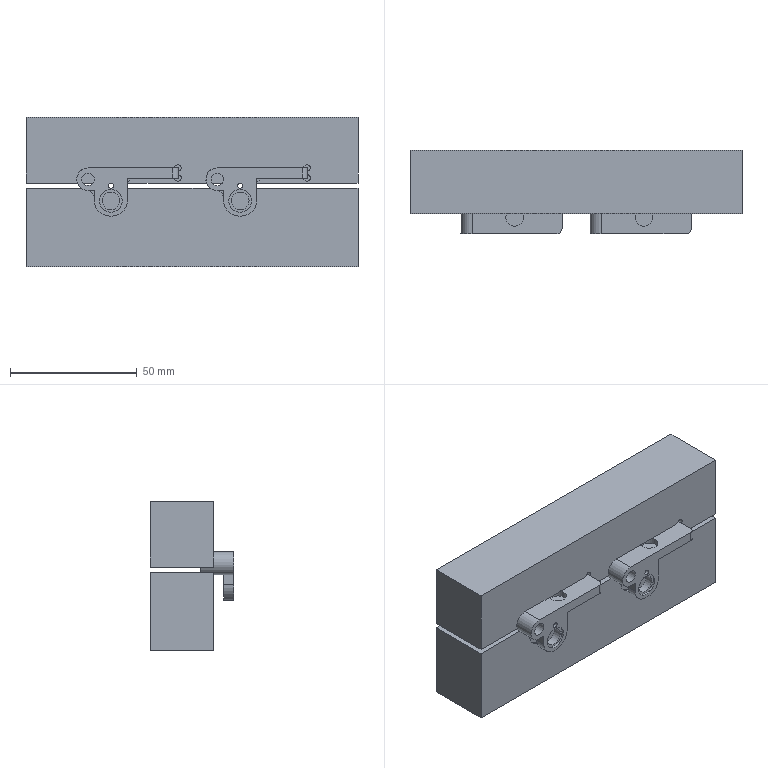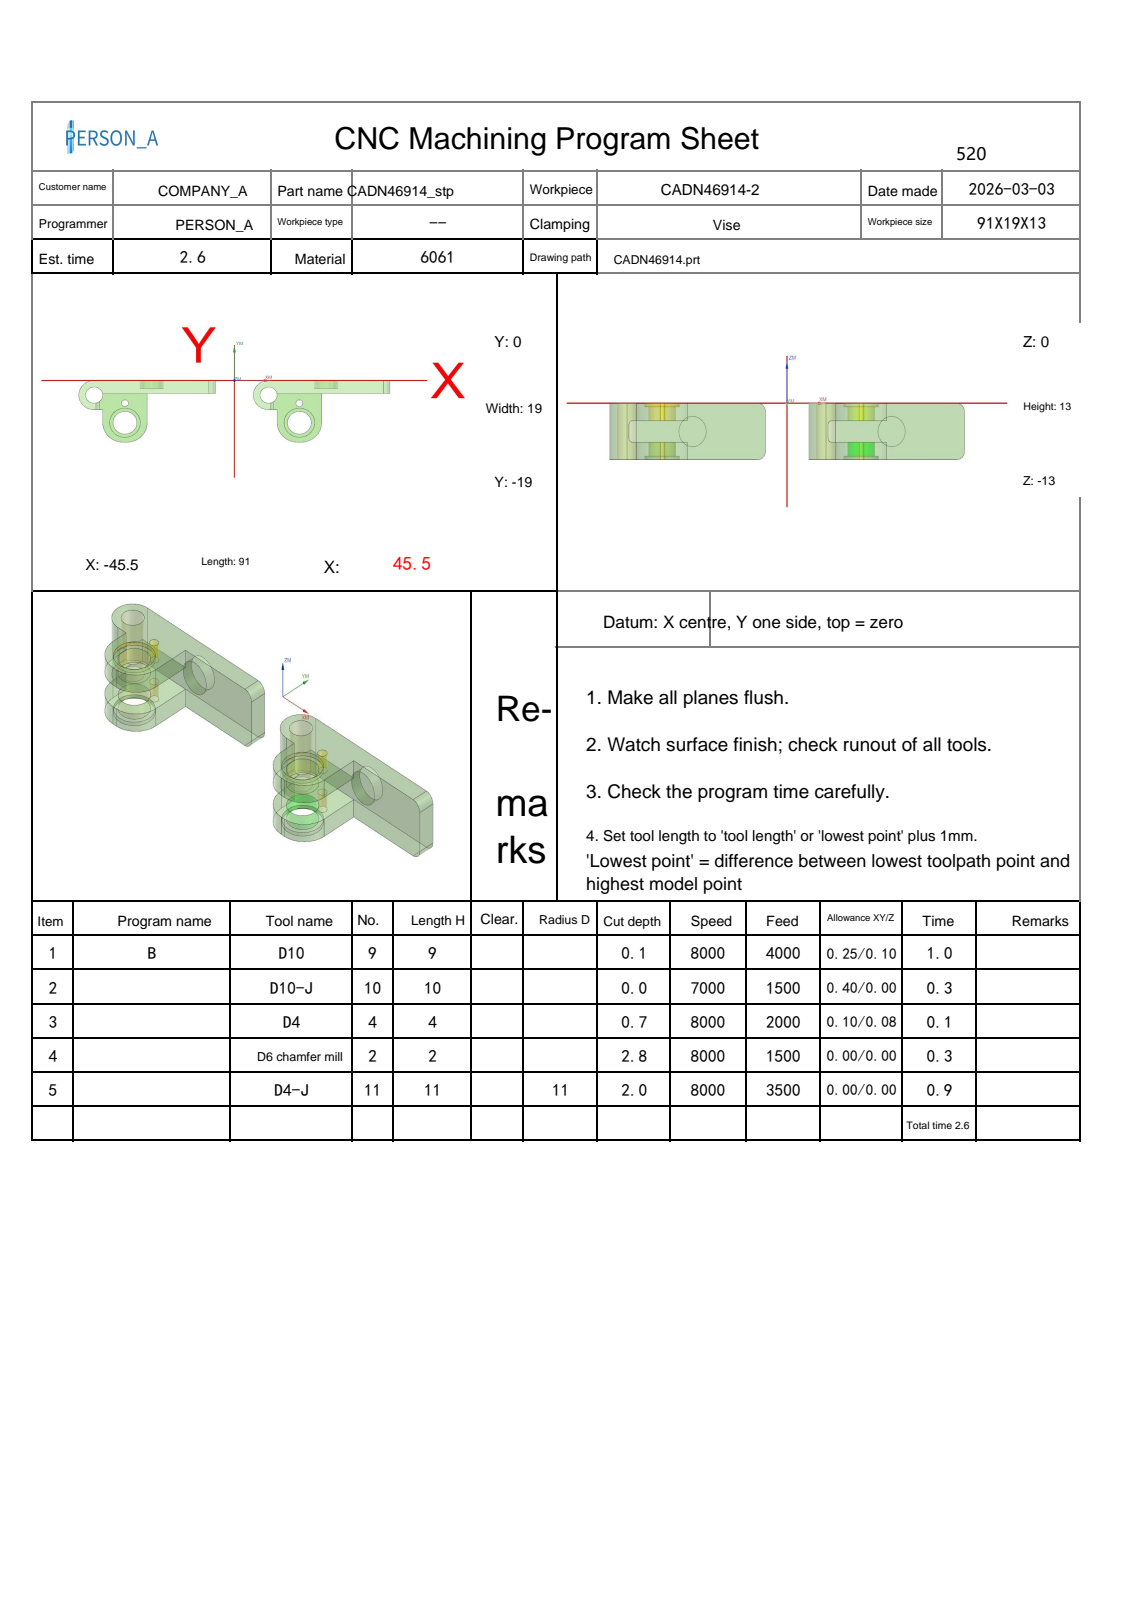NC program | NX | posted by the shop | part box 131 x 33 x 59 mm
Lines 824 to 1991 of 3834:
N5 T11 M06
(D4-J  D=4. R=0. H=11 ce=0.00 di=0.00)
G00 G90 G54 X20.661 Y-11.18 M03 S8000
G43 H11 Z50.
M08
Z.7
G01 X20.601 Y-11.119 Z.696 F600.
X20.28 Y-10.888 Z.675
X19.926 Y-10.71 Z.654
X19.549 Y-10.592 Z.633
X19.157 Y-10.535 Z.613
X18.843 Z.596
X18.451 Y-10.592 Z.575
X18.074 Y-10.71 Z.555
X17.72 Y-10.888 Z.534
X17.399 Y-11.119 Z.513
X17.119 Y-11.399 Z.492
X16.888 Y-11.72 Z.472
X16.71 Y-12.074 Z.451
X16.592 Y-12.451 Z.43
X16.535 Y-12.843 Z.409
Y-13.157 Z.393
X16.602 Y-13.593 Z.37
X16.746 Y-14.009 Z.347
X16.961 Y-14.394 Z.324
X17.241 Y-14.734 Z.301
X17.577 Y-15.019 Z.278
X17.959 Y-15.24 Z.254
X18.373 Y-15.389 Z.231
X18.808 Y-15.462 Z.208
X18.965 Y-15.465 Z.2
G41 D11
X19. Y-15.5
G03 X21.5 Y-13. Z-.05 I0.0 J2.5
X19. Y-10.5 Z-.3 I-2.5 J0.0
X16.5 Y-13. Z-.55 I0.0 J-2.5
X19. Y-15.5 Z-.8 I2.5 J0.0
X21.5 Y-13. I0.0 J2.5
X19. Y-10.5 I-2.5 J0.0
X16.5 Y-13. I0.0 J-2.5
X19. Y-15.5 I2.5 J0.0
X19.398 Y-15.468 I0.0 J2.5
G01 X19.425 Y-15.461
X19.442 Y-15.438
X19.44 Y-15.411
G40 X19.432 Y-15.361
Z.2
G00 Z50.
X-30.339 Y-11.18
Z.7
G01 X-30.399 Y-11.119 Z.696
X-30.72 Y-10.888 Z.675
X-31.074 Y-10.71 Z.654
X-31.451 Y-10.592 Z.633
X-31.843 Y-10.535 Z.613
X-32.157 Z.596
X-32.562 Y-10.595 Z.575
X-32.951 Y-10.721 Z.553
X-33.315 Y-10.909 Z.532
X-33.642 Y-11.155 Z.51
X-33.924 Y-11.452 Z.489
X-34.154 Y-11.791 Z.467
X-34.324 Y-12.163 Z.446
X-34.411 Y-12.465 Z.429
X-34.465 Y-12.843 Z.409
Y-13.157 Z.393
X-34.398 Y-13.593 Z.37
X-34.254 Y-14.009 Z.347
X-34.039 Y-14.394 Z.324
X-33.759 Y-14.734 Z.301
X-33.423 Y-15.019 Z.278
X-33.041 Y-15.24 Z.254
X-32.627 Y-15.389 Z.231
X-32.192 Y-15.462 Z.208
X-32.035 Y-15.465 Z.2
G41 D11
X-32. Y-15.5
G03 X-29.5 Y-13. Z-.05 I0.0 J2.5
X-32. Y-10.5 Z-.3 I-2.5 J0.0
X-34.401 Y-12.304 Z-.505 I0.0 J-2.5
X-34.5 Y-13. Z-.55 I2.401 J-.696
X-32. Y-15.5 Z-.8 I2.5 J0.0
X-29.5 Y-13. I0.0 J2.5
X-32. Y-10.5 I-2.5 J0.0
X-34.5 Y-13. I0.0 J-2.5
X-32. Y-15.5 I2.5 J0.0
X-31.602 Y-15.468 I0.0 J2.5
G01 X-31.575 Y-15.461
X-31.558 Y-15.438
X-31.56 Y-15.411
G40 X-31.568 Y-15.361
Z.2
G00 Z50.
G00 G90 X45.736 Y4.457 M03 S7000
Z11.8
Z.492
G01 Z-.008 F3500.
X45.531 Y1.1
X45.526 Y.932
G03 X45.689 Y0.0 I2.753 J0.0
G01 Y-4.
G03 X45.52 Y-5.003 I2.898 J-1.003
G01 X45.522 Y-5.1
X45.55 Z-.012
G02 X45.729 Y-4. I4.478 J-.164
G01 Y0.0
G02 X45.564 Y1.087 I3.504 J1.087
G01 Y1.1
X45.597 Z-.016
X45.589 Y.947
G03 X45.689 Y.432 I1.374 J0.0
G02 X45.762 Y.053 I-.937 J-.379
G01 Y-4.
X45.733 Y-4.291
G03 X45.578 Y-5.063 I1.838 J-.772
G01 Y-5.1
X45.606 Z-.02
X45.605 Y-5.046
G02 X45.748 Y-4.417 I1.453 J0.0
G01 X45.792 Y-4.
Y0.0
X45.748 Y.416
G02 X45.621 Y.951 I1.057 J.535
G01 X45.63 Y1.1
X45.663 Z-.024
X45.668 Y.971
X45.66 Y.811
X45.748 Y.528
G02 X45.819 Y0.0 I-4.089 J-.815
G01 Y-4.
X45.756 Y-4.489
X45.748 Y-4.525
G03 X45.633 Y-5.044 I1.112 J-.519
G01 X45.634 Y-5.1
X45.663 Z-.028
X45.662 Y-5.056
G02 X45.748 Y-4.634 I1.07 J0.0
G01 X45.843 Y-4.
Y0.0
G03 X45.72 Y.726 I-4.3 J-.357
G02 X45.688 Y.976 I.963 J.25
G01 X45.696 Y1.1
X45.726 Z-.03
X45.729 Z-.032
X45.724 Y.974
G03 X45.83 Y.38 I1.723 J0.0
G01 X45.808 Y.323
X45.817 Y.262
X45.855 Y.214
X45.866 Y0.0
Y-4.
G02 X45.748 Y-4.747 I-17.927 J2.45
G01 X45.711 Y-4.858
X45.691 Y-5.1
X45.719 Z-.036
X45.772 Y-4.693
G03 X45.888 Y-4. I-10.018 J2.037
G01 Y0.0
X45.874 Y.214
X45.837 Y.263
X45.829 Y.324
X45.851 Y.381
G02 X45.747 Y.936 I1.426 J.555
G01 X45.756 Y1.1
X45.774 Z-.04
X45.781 Y.67
X45.806 Y.569
X45.827 Y.536
G02 X45.871 Y.311 I-.552 J-.225
G01 X45.867 Y.244
X45.893 Y.214
X45.908 Y0.0
Y-4.
X45.833 Y-4.494
X45.815 Y-4.575
X45.809 Y-4.581
G03 X45.748 Y-5.1 I2.242 J-.523
G01 X45.763 Z-.044
G02 X45.87 Y-4.425 I2.314 J-.02
G01 X45.927 Y-4.
Y0.0
X45.912 Y.214
X45.887 Y.244
X45.891 Y.312
G03 X45.834 Y.555 I-.551 J0.0
G01 X45.822 Y.572
X45.795 Y.672
X45.792 Y1.101
X45.811 Z-.048
X45.81 Y.674
G02 X45.907 Y.384 I-5.292 J-1.938
G01 X45.886 Y.326
X45.895 Y.264
X45.931 Y.214
X45.946 Y0.0
Y-4.
X45.89 Y-4.426
G03 X45.777 Y-5.1 I2.008 J-.681
G01 X45.789 Z-.05
X45.792 Z-.052
Y-5.083
G02 X45.91 Y-4.428 I1.881 J0.0
G01 X45.963 Y-4.
Y0.0
X45.95 Y.214
X45.914 Y.264
X45.905 Y.326
X45.926 Y.385
G03 X45.824 Y.677 I-4.91 J-1.541
G01 X45.829 Y1.101
X45.847 Y1.102 Z-.056
X45.839 Y.66
X45.833 Y.629
X45.855 Y.608
G02 X45.951 Y.312 I-.411 J-.296
G01 X45.946 Y.244
X45.968 Y.214
X45.98 Y0.0
Y-4.
X45.937 Y-4.372
G02 X45.857 Y-4.628 I-.71 J.082
G01 X45.843 Y-4.704
X45.807 Y-5.1
X45.822 Z-.058
Z-.06
X45.857 Y-4.706
X45.872 Y-4.63
G03 X45.955 Y-4.376 I-.557 J.323
G01 X45.996 Y-4.
Y0.0
G03 X45.917 Y.55 I-2.783 J-.122
G01 X45.875 Y.581
X45.852 Y.629
X45.854 Y.681
X45.865 Y1.102
X45.884 Z-.064
X45.888 Y.971
G02 X45.871 Y.706 I-2.167 J0.0
G01 X45.864 Y.646
X45.887 Y.59
X45.934 Y.552
G02 X46.012 Y0.0 I-2.585 J-.645
G01 Y-4.
X45.964 Y-4.431
X45.948 Y-4.502
G03 X45.871 Y-4.708 I.656 J-.36
G01 X45.836 Y-5.1
X45.851 Z-.068
G03 X45.886 Y-4.736 I-1.913 J.364
G01 X45.885 Y-4.71
G02 X45.962 Y-4.503 I.999 J-.252
G01 X45.978 Y-4.432
X46.027 Y-4.
Y0.0
G03 X45.94 Y.572 I-2.104 J-.029
G01 X45.898 Y.595
X45.877 Y.638
X45.883 Y.686
G03 X45.902 Y.965 I-2.004 J.279
G01 X45.898 Y1.102
X45.91 Z-.072
X45.913 Y.968
G02 X45.898 Y.688 I-2.471 J0.0
G01 X45.892 Y.64
X45.915 Y.597
X45.958 Y.574
G02 X46.042 Y0.0 I-2.037 J-.592
G01 Y-4.
G02 X45.955 Y-4.575 I-2.129 J.026
G01 X45.917 Y-4.611
X45.897 Y-4.66
X45.9 Y-4.713
Y-4.738
G02 X45.866 Y-5.1 I-1.927 J0.0
G01 X45.88 Z-.076
G03 X45.914 Y-4.715 I-2.518 J.419
G01 X45.913 Y-4.661
X45.933 Y-4.612
X45.972 Y-4.575
G03 X46.056 Y-4. I-2.075 J.597
G01 Y0.0
G03 X45.971 Y.576 I-2.117 J-.018
G01 X45.949 Y.591
X45.912 Y.69
X45.922 Y1.101
X45.934 Z-.08
X45.927 Y.692
G02 X46.031 Y.392 I-1.015 J-.522
G01 X46.036 Y.36
X46.07 Y0.0
Y-4.
G02 X45.985 Y-4.575 I-2.222 J.034
G01 X45.949 Y-4.614
X45.929 Y-4.663
X45.928 Y-4.717
X45.894 Y-5.1
X45.908 Z-.084
X45.942 Y-4.719
X45.953 Y-4.64
X45.999 Y-4.575
G03 X46.084 Y-4. I-2.215 J.621
G01 Y0.0
G03 X46.04 Y.412 I-2.811 J-.092
X45.941 Y.694 I-.958 J-.175
G01 X45.946 Y1.101
X45.958 Z-.088
X45.956 Y.697
X46.026 Y.528
G02 X46.097 Y0.0 I-2.463 J-.6
G01 Y-4.
G02 X45.957 Y-4.721 I-2.033 J.02
G01 X45.922 Y-5.1
X45.935 Z-.09
X45.936 Z-.092
X45.971 Y-4.723
G03 X46.11 Y-4. I-1.992 J.757
G01 Y0.0
G03 X46.069 Y.364 I-1.998 J-.036
X45.971 Y.699 I-.938 J-.096
G01 X45.97 Y1.101
X45.982 Z-.096
X45.985 Y.701
G02 X46.122 Y0.0 I-1.796 J-.715
G01 Y-4.
G02 X45.985 Y-4.726 I-2.235 J.046
G01 X45.95 Y-5.1
X45.961 Z-.098
X45.964 Z-.1
X45.962 Y-5.047
G02 X46.023 Y-4.657 I1.28 J0.0
G03 X46.135 Y-4. I-2.24 J.717
G01 Y0.0
G03 X46. Y.703 I-2.075 J-.033
G02 X45.99 Y.942 I2.808 J.239
G01 X45.994 Y1.1
X46.006 Z-.104
X46. Y.946
G03 X46.014 Y.706 I2.056 J0.0
G02 X46.147 Y0.0 I-2.099 J-.758
G01 Y-4.
G02 X46.033 Y-4.672 I-2.456 J.07
G03 X45.976 Y-5.039 I1.161 J-.368
G01 X45.978 Y-5.1
X45.992 Z-.108
X45.991 Y-5.053
G02 X46.053 Y-4.631 I1.467 J0.0
G03 X46.158 Y-4. I-2.039 J.665
G01 Y0.0
G03 X46.051 Y.642 I-2.402 J-.073
G02 X46.005 Y.94 I.954 J.298
G01 X46.018 Y1.1
X46.03 Z-.112
X46.019 Y.944
G03 X46.068 Y.62 I1.099 J0.0
G02 X46.17 Y0.0 I-2.202 J-.68
G01 Y-4.
G02 X46.082 Y-4.575 I-2.064 J.021
G03 X46.004 Y-5.042 I1.367 J-.468
G01 X46.006 Y-5.1
X46.02 Z-.116
X46.017 Y-5.023
G02 X46.093 Y-4.575 I1.362 J0.0
G03 X46.181 Y-4. I-1.873 J.58
G01 Y0.0
G03 X46.081 Y.613 I-2.249 J-.055
G02 X46.03 Y.945 I1.066 J.331
G01 X46.041 Y1.1
X46.052 Z-.12
X46.041 Y.946
G03 X46.093 Y.608 I1.127 J0.0
G02 X46.193 Y0.0 I-2.066 J-.65
G01 Y-4.
Y-4.001
G02 X46.105 Y-4.575 I-1.915 J0.0
G03 X46.03 Y-5.005 I1.2 J-.43
G01 X46.034 Y-5.1
X46.047 Z-.124
X46.043 Y-4.994
G02 X46.117 Y-4.575 I1.225 J0.0
G03 X46.204 Y-4. I-1.881 J.581
G01 Y0.0
G03 X46.103 Y.612 I-2.103 J-.033
G02 X46.052 Y.941 I1.023 J.329
G01 X46.063 Y1.1
X46.074 Z-.127
X46.075 Z-.129
X46.064 Y.942
G03 X46.117 Y.606 I1.09 J0.0
G02 X46.216 Y0.0 I-1.934 J-.627
G01 Y-4.
G02 X46.129 Y-4.575 I-2.03 J.013
G01 X46.123 Y-4.605
G03 X46.063 Y-4.858 I.582 J-.272
G01 X46.061 Y-5.1
X46.075 Z-.133
Y-4.858
G02 X46.135 Y-4.607 I.561 J0.0
G01 X46.141 Y-4.575
G03 X46.227 Y-4. I-1.995 J.593
G01 Y0.0
G03 X46.127 Y.609 I-1.97 J-.011
G02 X46.074 Y.938 I.99 J.329
G01 X46.087 Y1.1
X46.098 Z-.137
X46.087 Y.94
G03 X46.141 Y.603 I1.075 J0.0
G02 X46.239 Y0.0 I-1.843 J-.609
G01 Y-4.
G02 X46.153 Y-4.575 I-2.122 J.022
G01 X46.146 Y-4.609
G03 X46.087 Y-4.844 I.439 J-.235
G01 X46.088 Y-4.858
X46.09 Y-5.1
X46.104 Z-.142
X46.096 Y-4.96
G02 X46.133 Y-4.66 I1.221 J0.0
G01 X46.134 Y-4.629
X46.158 Y-4.61
G03 X46.25 Y-4. I-2.17 J.639
G01 Y0.0
G03 X46.153 Y.602 I-1.912 J0.0
G02 X46.098 Y.94 I1.019 J.338
G01 X46.11 Y1.1
X46.122 Z-.146
X46.11 Y.939
G03 X46.165 Y.601 I1.067 J0.0
G02 X46.261 Y.007 I-1.782 J-.594
G01 Y0.0
Y-4.
G02 X46.17 Y-4.612 I-2.358 J.038
G01 X46.147 Y-4.625
Y-4.652
G03 X46.109 Y-4.951 I1.172 J-.299
G01 X46.118 Y-5.1
X46.133 Z-.151
X46.123 Y-4.941
G02 X46.158 Y-4.647 I1.281 J0.0
G01 X46.183 Y-4.614
X46.191 Y-4.575
G03 X46.273 Y-4. I-2.282 J.616
G01 Y0.0
Y.02
G03 X46.179 Y.598 I-1.819 J0.0
G02 X46.123 Y.939 I1.02 J.342
G01 X46.135 Y1.1
X46.148 Z-.156
X46.142 Y.95
G03 X46.163 Y.677 I1.825 J0.0
G01 X46.204 Y.567
G02 X46.285 Y0.0 I-2.027 J-.579
G01 Y-4.
G02 X46.205 Y-4.575 I-2.48 J.05
G01 X46.196 Y-4.616
X46.17 Y-4.649
G03 X46.138 Y-4.931 I1.237 J-.282
G01 X46.149 Y-5.099
X46.166 Z-.161
X46.153 Y-4.92
G02 X46.182 Y-4.65 I1.257 J0.0
G01 X46.207 Y-4.642
X46.209 Y-4.617
G03 X46.297 Y-4. I-2.501 J.672
G01 Y.001
G03 X46.227 Y.528 I-2.027 J0.0
G01 X46.214 Y.607
X46.175 Y.679
G02 X46.156 Y.95 I1.921 J.271
G01 X46.162 Y1.1
X46.176 Z-.166
X46.171 Y.95
G03 X46.188 Y.681 I2.08 J0.0
G01 X46.227 Y.608
X46.24 Y.528
X46.256 Y.461
G02 X46.309 Y0.0 I-2.192 J-.484
G01 Y-4.
G02 X46.223 Y-4.618 I-2.688 J.057
G01 X46.221 Y-4.644
X46.195 Y-4.652
G03 X46.168 Y-4.919 I1.285 J-.266
G01 X46.18 Y-5.099
X46.194 Z-.172
X46.183 Y-4.921
G02 X46.208 Y-4.654 I1.41 J0.0
G01 X46.233 Y-4.648
X46.235 Y-4.623
G03 X46.321 Y-4. I-2.561 J.671
G01 Y0.0
G03 X46.267 Y.463 I-2.145 J-.015
G01 X46.253 Y.528
X46.241 Y.61
X46.201 Y.682
G02 X46.185 Y.951 I2.241 J.268
G01 X46.19 Y1.1
X46.205 Z-.177
X46.2 Y.951
G03 X46.215 Y.684 I2.482 J0.0
G01 X46.252 Y.612
X46.265 Y.528
X46.293 Y.394
G02 X46.333 Y.004 I-1.891 J-.39
G01 Y0.0
Y-4.
G02 X46.257 Y-4.575 I-2.517 J.039
G01 X46.25 Y-4.624
X46.221 Y-4.656
G03 X46.198 Y-4.923 I1.506 J-.267
G01 X46.208 Y-5.099
X46.222 Y-5.1 Z-.183
X46.213 Y-4.926
G02 X46.235 Y-4.658 I1.677 J0.0
G01 X46.26 Y-4.625
X46.268 Y-4.575
G03 X46.345 Y-4. I-2.36 J.611
G01 Y0.0
G03 X46.306 Y.396 I-2.002 J-.001
G01 X46.276 Y.528
X46.262 Y.613
X46.228 Y.686
X46.22 Y1.1
X46.235 Z-.188
X46.242 Y.688
G02 X46.358 Y.026 I-1.839 J-.662
G01 X46.357 Y0.0
Y-4.
G02 X46.278 Y-4.575 I-2.392 J.036
G01 X46.27 Y-4.627
X46.249 Y-4.66
G03 X46.229 Y-4.929 I1.844 J-.269
G01 X46.237 Y-5.1
X46.252 Z-.194
X46.243 Y-4.936
G02 X46.289 Y-4.575 I1.424 J0.0
G03 X46.37 Y-4. I-2.353 J.623
G01 Y0.0
G03 X46.257 Y.69 I-2.423 J-.044
G01 X46.25 Y1.1
X46.266 Z-.2
X46.271 Y.692
G02 X46.382 Y0.0 I-2.573 J-.768
G01 Y-4.
G02 X46.277 Y-4.664 I-2.581 J.068
G01 X46.268 Y-4.736
X46.267 Y-5.1
X46.283 Z-.206
X46.284 Y-4.738
X46.292 Y-4.666
G03 X46.394 Y-4. I-2.777 J.769
G01 Y0.0
G03 X46.34 Y.449 I-2.024 J-.018
G02 X46.275 Y.945 I1.877 J.496
G01 X46.282 Y1.1
X46.297 Z-.209
X46.298 Z-.212
X46.292 Y.942
G03 X46.355 Y.425 I2.135 J0.0
G02 X46.407 Y.009 I-1.672 J-.417
G01 Y-4.
G02 X46.365 Y-4.39 I-2.247 J.04
G01 X46.323 Y-4.575
X46.307 Y-4.669
X46.298 Y-5.1
X46.314 Z-.218
X46.313 Y-4.984
G02 X46.334 Y-4.575 I3.849 J0.0
G01 X46.377 Y-4.392
G03 X46.419 Y-4. I-2.138 J.426
G01 Y.002
G03 X46.381 Y.357 I-1.708 J0.0
G01 X46.345 Y.528
G02 X46.311 Y.957 I2.652 J.43
G01 X46.315 Y1.1
X46.326 Z-.225
X46.323 Y.959
G03 X46.357 Y.528 I2.726 J0.0
G01 X46.398 Y.333
G02 X46.431 Y.015 I-1.506 J-.318
G01 Y-4.
G02 X46.389 Y-4.393 I-2.101 J.026
G01 X46.346 Y-4.575
G03 X46.324 Y-4.985 I3.841 J-.41
G01 X46.326 Y-5.1
X46.338 Z-.231
X46.336 Y-4.985
G02 X46.358 Y-4.575 I3.863 J0.0
G01 X46.401 Y-4.394
G03 X46.443 Y-4. I-1.974 J.411
G01 Y.004
G03 X46.4 Y.379 I-1.651 J0.0
G02 X46.334 Y.955 I2.469 J.576
G01 X46.338 Y1.1
X46.35 Z-.238
X46.346 Y.955
G03 X46.414 Y.37 I2.558 J0.0
G02 X46.456 Y.011 I-1.528 J-.359
G01 Y-4.
G02 X46.37 Y-4.575 I-2.16 J.026
G03 X46.349 Y-4.985 I3.841 J-.41
G01 X46.35 Y-5.1
X46.363 Z-.244
X46.361 Y-4.985
G02 X46.383 Y-4.575 I3.863 J0.0
G01 X46.426 Y-4.397
G03 X46.468 Y-4. I-2.625 J.477
G01 Y.047
G03 X46.408 Y.453 I-1.405 J0.0
G02 X46.359 Y.955 I2.534 J.502
G01 X46.363 Y1.1
X46.375 Z-.251
X46.371 Y.955
G03 X46.42 Y.454 I2.609 J0.0
G02 X46.48 Y.063 I-1.24 J-.391
G01 Y-4.
Y-4.013
G02 X46.439 Y-4.398 I-1.822 J0.0
G01 X46.395 Y-4.575
G03 X46.374 Y-4.985 I3.841 J-.41
G01 X46.375 Y-5.1
X46.388 Z-.258
X46.386 Y-4.985
G02 X46.408 Y-4.575 I3.863 J0.0
G01 X46.438 Y-4.454
G03 X46.492 Y-4.013 I-1.772 J.441
G01 Y.079
G03 X46.432 Y.455 I-1.203 J0.0
G01 X46.417 Y.528
G02 X46.384 Y.96 I2.832 J.432
G01 X46.388 Y1.1
X46.401 Z-.265
X46.397 Y.96
G03 X46.43 Y.528 I2.893 J0.0
G01 X46.444 Y.455
G02 X46.504 Y.073 I-1.191 J-.383
G01 Y-4.
G02 X46.443 Y-4.49 I-1.978 J0.0
G01 X46.421 Y-4.575
G03 X46.399 Y-4.985 I3.841 J-.41
G01 X46.401 Y-5.1
X46.414 Z-.272
X46.412 Y-4.985
G02 X46.434 Y-4.575 I3.863 J0.0
G01 X46.456 Y-4.488
G03 X46.516 Y-4. I-2.07 J.504
G01 Y.065
G03 X46.457 Y.456 I-1.315 J0.0
G01 X46.443 Y.528
G02 X46.411 Y.96 I2.892 J.432
G01 X46.414 Y1.1
X46.427 Z-.279
X46.424 Y.96
G03 X46.456 Y.528 I2.959 J0.0
G01 X46.469 Y.457
G02 X46.528 Y.057 I-1.322 J-.4
G01 Y-4.
G02 X46.456 Y-4.54 I-2.211 J.022
G01 X46.447 Y-4.575
G03 X46.425 Y-4.985 I3.838 J-.41
G01 X46.427 Y-5.1
X46.44 Z-.286
X46.439 Y-4.985
G02 X46.46 Y-4.575 I3.884 J0.0
G01 X46.493 Y-4.432
G03 X46.54 Y-4. I-2.126 J.449
G01 Y.051
G03 X46.482 Y.458 I-1.45 J0.0
G02 X46.437 Y.956 I2.713 J.498
G01 X46.44 Y1.1
X46.454 Z-.293
X46.45 Y.956
G03 X46.495 Y.459 I2.792 J0.0
G02 X46.552 Y.038 I-1.515 J-.421
G01 Y-4.
G02 X46.505 Y-4.433 I-2.117 J.01
G01 X46.474 Y-4.575
G03 X46.452 Y-4.985 I3.925 J-.41
G01 X46.454 Y-5.1
X46.468 Z-.3
X46.466 Y-4.985
G02 X46.487 Y-4.575 I4.012 J0.0
G01 X46.518 Y-4.434
G03 X46.564 Y-4. I-2.139 J.449
G01 Y.002
G03 X46.526 Y.369 I-1.769 J0.0
G02 X46.464 Y.957 I2.766 J.587
G01 X46.468 Y1.1
X46.482 Z-.308
X46.478 Y.957
G03 X46.539 Y.369 I2.866 J0.0
G02 X46.576 Y.01 I-1.71 J-.358
G01 Y-4.
G02 X46.53 Y-4.435 I-2.362 J.03
G01 X46.501 Y-4.575
G03 X46.48 Y-4.985 I4.061 J-.411
G01 X46.482 Y-5.1
X46.496 Z-.316
X46.492 Y-4.948
G02 X46.543 Y-4.436 I2.581 J0.0
G03 X46.588 Y-4. I-2.505 J.481
G01 Y.002
G03 X46.55 Y.38 I-1.906 J0.0
G02 X46.492 Y.957 I2.848 J.577
G01 X46.496 Y1.1
X46.51 Z-.323
X46.507 Y.961
G03 X46.567 Y.351 I3.179 J0.0
G02 X46.6 Y.003 I-1.778 J-.348
G01 Y-4.
G02 X46.556 Y-4.437 I-2.899 J.074
G03 X46.506 Y-4.95 I2.634 J-.513
G01 X46.511 Y-5.1
X46.525 Z-.331
X46.521 Y-4.952
G02 X46.569 Y-4.438 I2.799 J0.0
G03 X46.612 Y-4. I-3.667 J.584
G01 Y.003
G03 X46.579 Y.361 I-1.922 J0.0
G02 X46.522 Y.961 I3.165 J.6
G01 X46.525 Y1.1
X46.54 Z-.339
X46.537 Y.961
G03 X46.592 Y.366 I3.266 J0.0
G02 X46.624 Y.013 I-1.903 J-.353
G01 Y-4.
G02 X46.582 Y-4.439 I-3.496 J.113
G03 X46.536 Y-4.954 I2.884 J-.515
G01 X46.54 Y-5.1
X46.555 Z-.347
X46.552 Y-4.957
G02 X46.595 Y-4.44 I3.081 J0.0
G03 X46.636 Y-4. I-5.131 J.694
G01 Y0.0
G03 X46.59 Y.472 I-3.842 J-.137
G02 X46.551 Y.955 I3.011 J.483
G01 X46.555 Y1.1
X46.57 Z-.355
X46.567 Y.962
G03 X46.595 Y.528 I3.359 J0.0
G02 X46.648 Y0.0 I-4.997 J-.763
G01 Y-4.
G02 X46.601 Y-4.482 I-5.573 J.296
G03 X46.568 Y-4.963 I3.414 J-.48
G01 X46.57 Y-5.1
X46.586 Z-.363
X46.601 Y-4.575
G03 X46.66 Y-4. I-6.939 J1.002
G01 Y0.0
X46.652 Y.122
X46.597 Y.605
X46.586 Y1.1
X46.6 Z-.372
X46.598 Y.961
G03 X46.616 Y.528 I5.152 J0.0
G01 X46.653 Y.244
X46.671 Y0.0
Y-4.
G02 X46.611 Y-4.575 I-6.521 J.396
G03 X46.599 Y-4.986 I7.114 J-.411
G01 X46.6 Y-5.1
X46.601 Z-.376
X46.61 Z-.38
X46.621 Y-4.575
G03 X46.683 Y-4. I-5.961 J.933
G01 Y0.0
X46.665 Y.244
X46.627 Y.528
G02 X46.608 Y.962 I5.145 J.434
G01 X46.61 Y1.1
X46.614 Z-.385
X46.621 Z-.389
X46.619 Y.962
G03 X46.637 Y.528 I5.171 J0.0
G01 X46.677 Y.244
X46.695 Y0.0
Y-4.
G02 X46.632 Y-4.575 I-5.525 J.317
G01 X46.621 Y-5.1
X46.631 Z-.397
X46.642 Y-4.575
G03 X46.706 Y-4. I-4.984 J.849
G01 Y0.0
X46.689 Y.244
X46.647 Y.528
G02 X46.629 Y.962 I5.159 J.434
G01 X46.631 Y1.1
X46.642 Z-.406
X46.64 Y.962
G03 X46.658 Y.528 I5.185 J0.0
G01 X46.701 Y.244
X46.718 Y0.0
Y-4.
G02 X46.653 Y-4.575 I-4.601 J.232
G01 X46.642 Y-5.1
X46.653 Z-.415
X46.663 Y-4.575
G03 X46.73 Y-4. I-4.12 J.765
G01 Y0.0
X46.713 Y.244
X46.669 Y.528
G02 X46.651 Y.962 I5.173 J.435
G01 X46.652 Y1.1
X46.663 Z-.424
X46.661 Y.962
G03 X46.68 Y.528 I5.199 J0.0
G01 X46.725 Y.244
X46.741 Y0.0
Y-4.
G02 X46.674 Y-4.575 I-3.807 J.151
G01 X46.663 Y-5.1
X46.674 Z-.433
X46.685 Y-4.575
G03 X46.752 Y-4. I-3.398 J.689
G01 Y0.0
X46.737 Y.244
X46.691 Y.528
G02 X46.672 Y.962 I5.188 J.435
G01 X46.674 Y1.1
X46.685 Z-.442
X46.683 Y.962
G03 X46.702 Y.528 I5.214 J0.0
G01 X46.748 Y.244
X46.764 Y0.0
Y-4.
G02 X46.696 Y-4.575 I-3.322 J.099
G01 X46.685 Y-5.1
X46.696 Z-.451
X46.707 Y-4.575
G03 X46.775 Y-4. I-3.486 J.702
G01 Y0.0
X46.758 Y.244
X46.713 Y.528
G02 X46.695 Y.963 I5.219 J.435
G01 X46.696 Y1.1
X46.708 Z-.46
X46.706 Y.963
G03 X46.724 Y.528 I5.244 J0.0
G01 X46.769 Y.244
X46.786 Y0.0
Y-4.
G02 X46.719 Y-4.575 I-3.795 J.156
G01 X46.708 Y-5.1
X46.719 Z-.469
X46.73 Y-4.575
G03 X46.797 Y-4. I-3.975 J.758
G01 Y0.0
X46.78 Y.244
X46.735 Y.528
G02 X46.717 Y.962 I5.215 J.435
G01 X46.719 Y1.1
X46.73 Z-.479
X46.729 Y.962
G03 X46.747 Y.528 I5.242 J0.0
G01 X46.79 Y.244
X46.808 Y0.0
Y-4.
G02 X46.741 Y-4.575 I-4.292 J.21
G01 X46.731 Y-5.1
X46.742 Z-.488
X46.753 Y-4.575
G03 X46.819 Y-4. I-4.471 J.809
G01 Y0.0
X46.801 Y.244
X46.758 Y.528
G02 X46.74 Y.962 I5.232 J.435
G01 X46.742 Y1.1
X46.754 Z-.498
X46.752 Y.962
G03 X46.77 Y.528 I5.258 J0.0
G01 X46.812 Y.244
X46.83 Y0.0
Y-4.
G02 X46.765 Y-4.575 I-4.771 J.256
G01 X46.754 Y-5.1
X46.766 Z-.508
X46.776 Y-4.575
G03 X46.841 Y-4. I-4.921 J.848
G01 Y0.0
X46.823 Y.244
X46.782 Y.528
G02 X46.764 Y.962 I5.248 J.435
G01 X46.766 Y1.1
X46.777 Z-.517
X46.776 Y.963
G03 X46.794 Y.528 I5.273 J0.0
G01 X46.834 Y.244
X46.852 Y0.0
Y-4.
G02 X46.788 Y-4.575 I-5.172 J.285
G01 X46.777 Y-5.1
X46.79 Z-.527
X46.8 Y-4.575
G03 X46.863 Y-4. I-5.263 J.866
G01 Y0.0
X46.846 Y.244
X46.806 Y.528
G02 X46.788 Y.963 I5.264 J.435
G01 X46.789 Y1.1
X46.802 Z-.537
X46.8 Y.963
G03 X46.818 Y.528 I5.309 J0.0
G01 X46.857 Y.244
X46.874 Y0.0
Y-4.
G02 X46.812 Y-4.575 I-5.431 J.29
G01 X46.802 Y-5.1
X46.814 Z-.547
X46.825 Y-4.575
G03 X46.884 Y-4. I-5.501 J.864
G01 Y0.0
G03 X46.869 Y.244 I-18.257 J-1.064
G01 X46.83 Y.528
G02 X46.812 Y.963 I5.3 J.436
G01 X46.814 Y1.1
X46.826 Z-.557
X46.824 Y.963
G03 X46.842 Y.528 I5.307 J0.0
G01 X46.88 Y.244
G02 X46.895 Y0.0 I-20.873 J-1.397
G01 Y-4.
G02 X46.837 Y-4.575 I-5.846 J.302
G01 X46.826 Y-5.1
X46.839 Z-.567
X46.849 Y-4.575
G03 X46.906 Y-4. I-5.903 J.868
G01 Y0.0
G03 X46.881 Y.282 I-3.599 J-.178
G02 X46.837 Y.963 I5.291 J.681
G01 X46.839 Y1.1
X46.851 Z-.578
X46.847 Y.928
G03 X46.88 Y.429 I3.767 J0.0
G01 X46.916 Y0.0
Y-4.
X46.862 Y-4.575
X46.851 Y-5.1
X46.864 Z-.588
G02 X46.927 Y-4. I10.127 J-.025
G01 Y0.0
X46.88 Y.528
G02 X46.862 Y.963 I5.334 J.436
G01 X46.864 Y1.1
X46.877 Z-.599
X46.88 Y.639
X46.889 Y.528
X46.937 Y0.0
Y-4.
G03 X46.877 Y-5.049 I9.083 J-1.049
G01 Y-5.1
X46.88 Z-.604
X46.887 Z-.609
X46.893 Y-4.575
X46.947 Y-4.
Y0.0
X46.91 Y.387
G02 X46.884 Y.939 I5.81 J.552
G01 X46.886 Y1.1
X46.895 Z-.62
X46.894 Y.963
G03 X46.906 Y.528 I7.963 J0.0
G02 X46.957 Y0.0 I-6.327 J-.887
G01 Y-4.
X46.902 Y-4.575
X46.896 Y-5.1
X46.905 Z-.63
X46.91 Y-4.575
X46.968 Y-4.
Y0.0
G03 X46.914 Y.528 I-5.745 J-.314
G02 X46.902 Y.963 I7.885 J.435
G01 X46.903 Y1.1
X46.912 Z-.641
X46.911 Y.963
G03 X46.923 Y.528 I7.833 J0.0
G02 X46.978 Y0.0 I-5.108 J-.796
G01 Y-4.
X46.919 Y-4.575
X46.914 Y-5.1
X46.923 Z-.652
X46.928 Y-4.575
G03 X46.988 Y-4. I-7.507 J1.072
G01 Y0.0
G03 X46.932 Y.528 I-4.635 J-.224
G02 X46.92 Y.962 I7.757 J.435
G01 X46.921 Y1.1
X46.929 Z-.663
X46.928 Y.962
G03 X46.941 Y.528 I7.705 J0.0
G02 X46.997 Y0.0 I-4.107 J-.71
G01 Y-4.
G02 X46.936 Y-4.575 I-6.561 J.405
G01 X46.932 Y-5.1
X46.941 Z-.674
X46.945 Y-4.575
G03 X47.007 Y-4. I-5.669 J.902
G01 Y0.0
G03 X46.949 Y.528 I-3.746 J-.144
G02 X46.937 Y.962 I7.63 J.434
G01 X46.938 Y1.1
X46.947 Z-.685
X46.946 Y.962
G03 X46.958 Y.528 I7.58 J0.0
G02 X47.017 Y0.0 I-3.319 J-.636
G01 Y-4.
G02 X46.954 Y-4.575 I-5.04 J.26
G01 X46.951 Y-5.1
X46.96 Z-.696
G02 X46.956 Y-4.874 I6.544 J.226
X46.963 Y-4.575 I6.548 J0.0
G03 X47.027 Y-4. I-4.398 J.778
G01 Y0.0
G03 X46.967 Y.528 I-3.052 J-.076
G02 X46.955 Y.962 I7.506 J.434
G01 X46.956 Y1.1
X46.965 Z-.708
X46.964 Y.961
G03 X46.976 Y.528 I7.458 J0.0
G02 X47.036 Y0.0 I-2.706 J-.574
G01 Y-4.
G02 X46.972 Y-4.575 I-3.973 J.153
G03 X46.965 Y-4.866 I6.22 J-.291
X46.97 Y-5.1 I6.226 J0.0
G01 X46.979 Z-.719
G02 X46.974 Y-4.859 I5.928 J.24
X46.981 Y-4.575 I5.933 J0.0
G03 X47.046 Y-4. I-3.663 J.703
G01 Y0.0
G03 X46.986 Y.528 I-2.921 J-.067
G02 X46.973 Y.961 I7.384 J.434
G01 X46.974 Y1.1
X46.983 Z-.73
X46.982 Y.961
G03 X46.995 Y.528 I7.337 J0.0
G02 X47.055 Y0.0 I-3.049 J-.617
G01 Y-4.
G02 X46.99 Y-4.575 I-3.963 J.157
G03 X46.983 Y-4.853 I5.657 J-.278
X46.989 Y-5.1 I5.664 J0.0
G01 X46.998 Z-.742
G02 X46.993 Y-4.847 I5.411 J.252
X46.999 Y-4.575 I5.417 J0.0
G03 X47.065 Y-4. I-4.138 J.76
G01 Y0.0
G03 X47.004 Y.528 I-3.301 J-.112
G02 X46.991 Y.961 I7.265 J.433
G01 X46.992 Y1.1
X47.002 Z-.753
X47. Y.961
G03 X47.013 Y.528 I7.219 J0.0
G02 X47.074 Y0.0 I-3.433 J-.662
G01 Y-4.
G02 X47.009 Y-4.575 I-4.442 J.213
G03 X47.002 Y-4.842 I5.183 J-.267
X47.008 Y-5.1 I5.19 J0.0
G01 X47.018 Z-.765
G02 X47.011 Y-4.837 I4.972 J.263
X47.018 Y-4.575 I4.979 J0.0
G03 X47.083 Y-4. I-4.611 J.813
G01 Y0.0
G03 X47.023 Y.528 I-3.682 J-.154
G02 X47.009 Y.961 I7.148 J.433
G01 X47.011 Y1.1
X47.02 Z-.777
X47.019 Y.96
G03 X47.032 Y.528 I7.103 J0.0
G02 X47.092 Y0.0 I-3.801 J-.7
G01 Y-4.
G02 X47.048 Y-4.445 I-4.898 J.262
G03 X47.018 Y-4.862 I2.86 J-.416
X47.028 Y-5.1 I2.89 J0.0
G01 X47.037 Z-.788
G02 X47.026 Y-4.856 I2.764 J.244
X47.055 Y-4.456 I2.775 J0.0
G03 X47.101 Y-4. I-5.055 J.737
G01 Y0.0
G03 X47.041 Y.528 I-4.025 J-.188
G02 X47.028 Y.96 I7.033 J.433
G01 X47.03 Y1.1
X47.035 Z-.8
X47.034 Y.96
G03 X47.047 Y.528 I7.014 J0.0
G02 X47.106 Y0.0 I-4.05 J-.722
G01 Y-4.
G02 X47.061 Y-4.456 I-5.205 J.29
G03 X47.032 Y-4.855 I2.758 J-.399
X47.043 Y-5.1 I2.786 J0.0
G01 X47.053 Z-.806
X47.057 Z-.812
G02 X47.046 Y-4.853 I2.801 J.247
X47.074 Y-4.457 I2.812 J0.0
G03 X47.119 Y-4. I-5.374 J.763
G01 Y0.0
G03 X47.061 Y.528 I-4.283 J-.206
G02 X47.047 Y.96 I6.921 J.432
G01 X47.049 Y1.1
X47.058 Z-.824
X47.057 Y.96
G03 X47.07 Y.528 I6.879 J0.0
G02 X47.128 Y0.0 I-4.308 J-.736
G01 Y-4.
G02 X47.083 Y-4.458 I-5.52 J.309
G03 X47.055 Y-4.851 I2.8 J-.393
X47.066 Y-5.1 I2.828 J0.0
G01 X47.076 Z-.836
G02 X47.065 Y-4.849 I2.83 J.25
X47.092 Y-4.46 I2.841 J0.0
G03 X47.136 Y-4. I-5.531 J.766
G01 Y0.0
G03 X47.08 Y.528 I-4.41 J-.205
G02 X47.066 Y.96 I6.81 J.432
G01 X47.068 Y1.1
X47.077 Z-.848
X47.076 Y.96
G03 X47.09 Y.528 I6.77 J0.0
G02 X47.145 Y0.0 I-4.36 J-.723
G01 Y-4.
G02 X47.102 Y-4.459 I-5.581 J.296
G03 X47.075 Y-4.849 I2.862 J-.39
X47.086 Y-5.1 I2.888 J0.0
G01 X47.096 Z-.86
G02 X47.085 Y-4.847 I2.886 J.253
X47.111 Y-4.46 I2.897 J0.0
G03 X47.154 Y-4. I-5.496 J.74
G01 Y0.0
X47.137 Y.244
X47.1 Y.528
G02 X47.086 Y.959 I6.702 J.432
G01 X47.087 Y1.1
X47.097 Z-.873
X47.095 Y.959
G03 X47.109 Y.528 I6.663 J0.0
G01 X47.146 Y.244
X47.162 Y0.0
Y-4.
G02 X47.12 Y-4.462 I-5.448 J.258
G03 X47.095 Y-4.845 I2.878 J-.383
X47.106 Y-5.1 I2.904 J0.0
G01 X47.113 Z-.879
X47.116 Z-.885
G02 X47.105 Y-4.843 I2.904 J.257
X47.129 Y-4.465 I2.915 J0.0
G03 X47.17 Y-4. I-5.492 J.717
G01 Y0.0
G03 X47.155 Y.244 I-15.808 J-.861
G01 X47.119 Y.528
G02 X47.105 Y.959 I6.603 J.432
G01 X47.107 Y1.1
X47.117 Z-.897
X47.115 Y.96
G03 X47.129 Y.528 I6.576 J0.0
G01 X47.163 Y.259
G02 X47.179 Y.002 I-2.079 J-.257
G01 Y-4.
G02 X47.139 Y-4.468 I-5.403 J.224
G03 X47.115 Y-4.841 I2.896 J-.373
X47.126 Y-5.1 I2.92 J0.0
G01 X47.134 Z-.91
G02 X47.125 Y-4.854 I3.198 J.245
X47.149 Y-4.462 I3.207 J0.0
G03 X47.187 Y-4. I-5.65 J.696
G01 Y0.0
G03 X47.154 Y.41 I-4.713 J-.17
G01 X47.139 Y.528
G02 X47.125 Y.96 I6.52 J.432
G01 X47.127 Y1.1
X47.137 Z-.922
X47.135 Y.956
G03 X47.157 Y.442 I6.011 J0.0
G01 X47.195 Y0.0
Y-4.